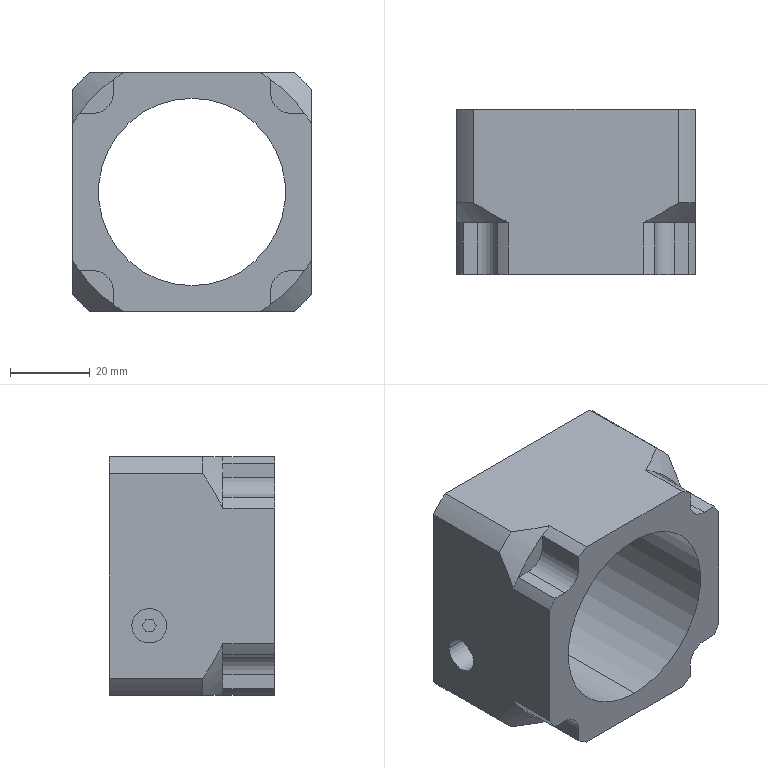Part | NX | 1 solid | 76 faces | box 60 x 41.5 x 60 mm | volume 68790 mm3 | plane 30 | cylinder 30 | cone 14 | torus 2 | commonest cylinder face diameters 3.3 x8 69 x8 10 x4 79 x4 8.7 x2 47 x2